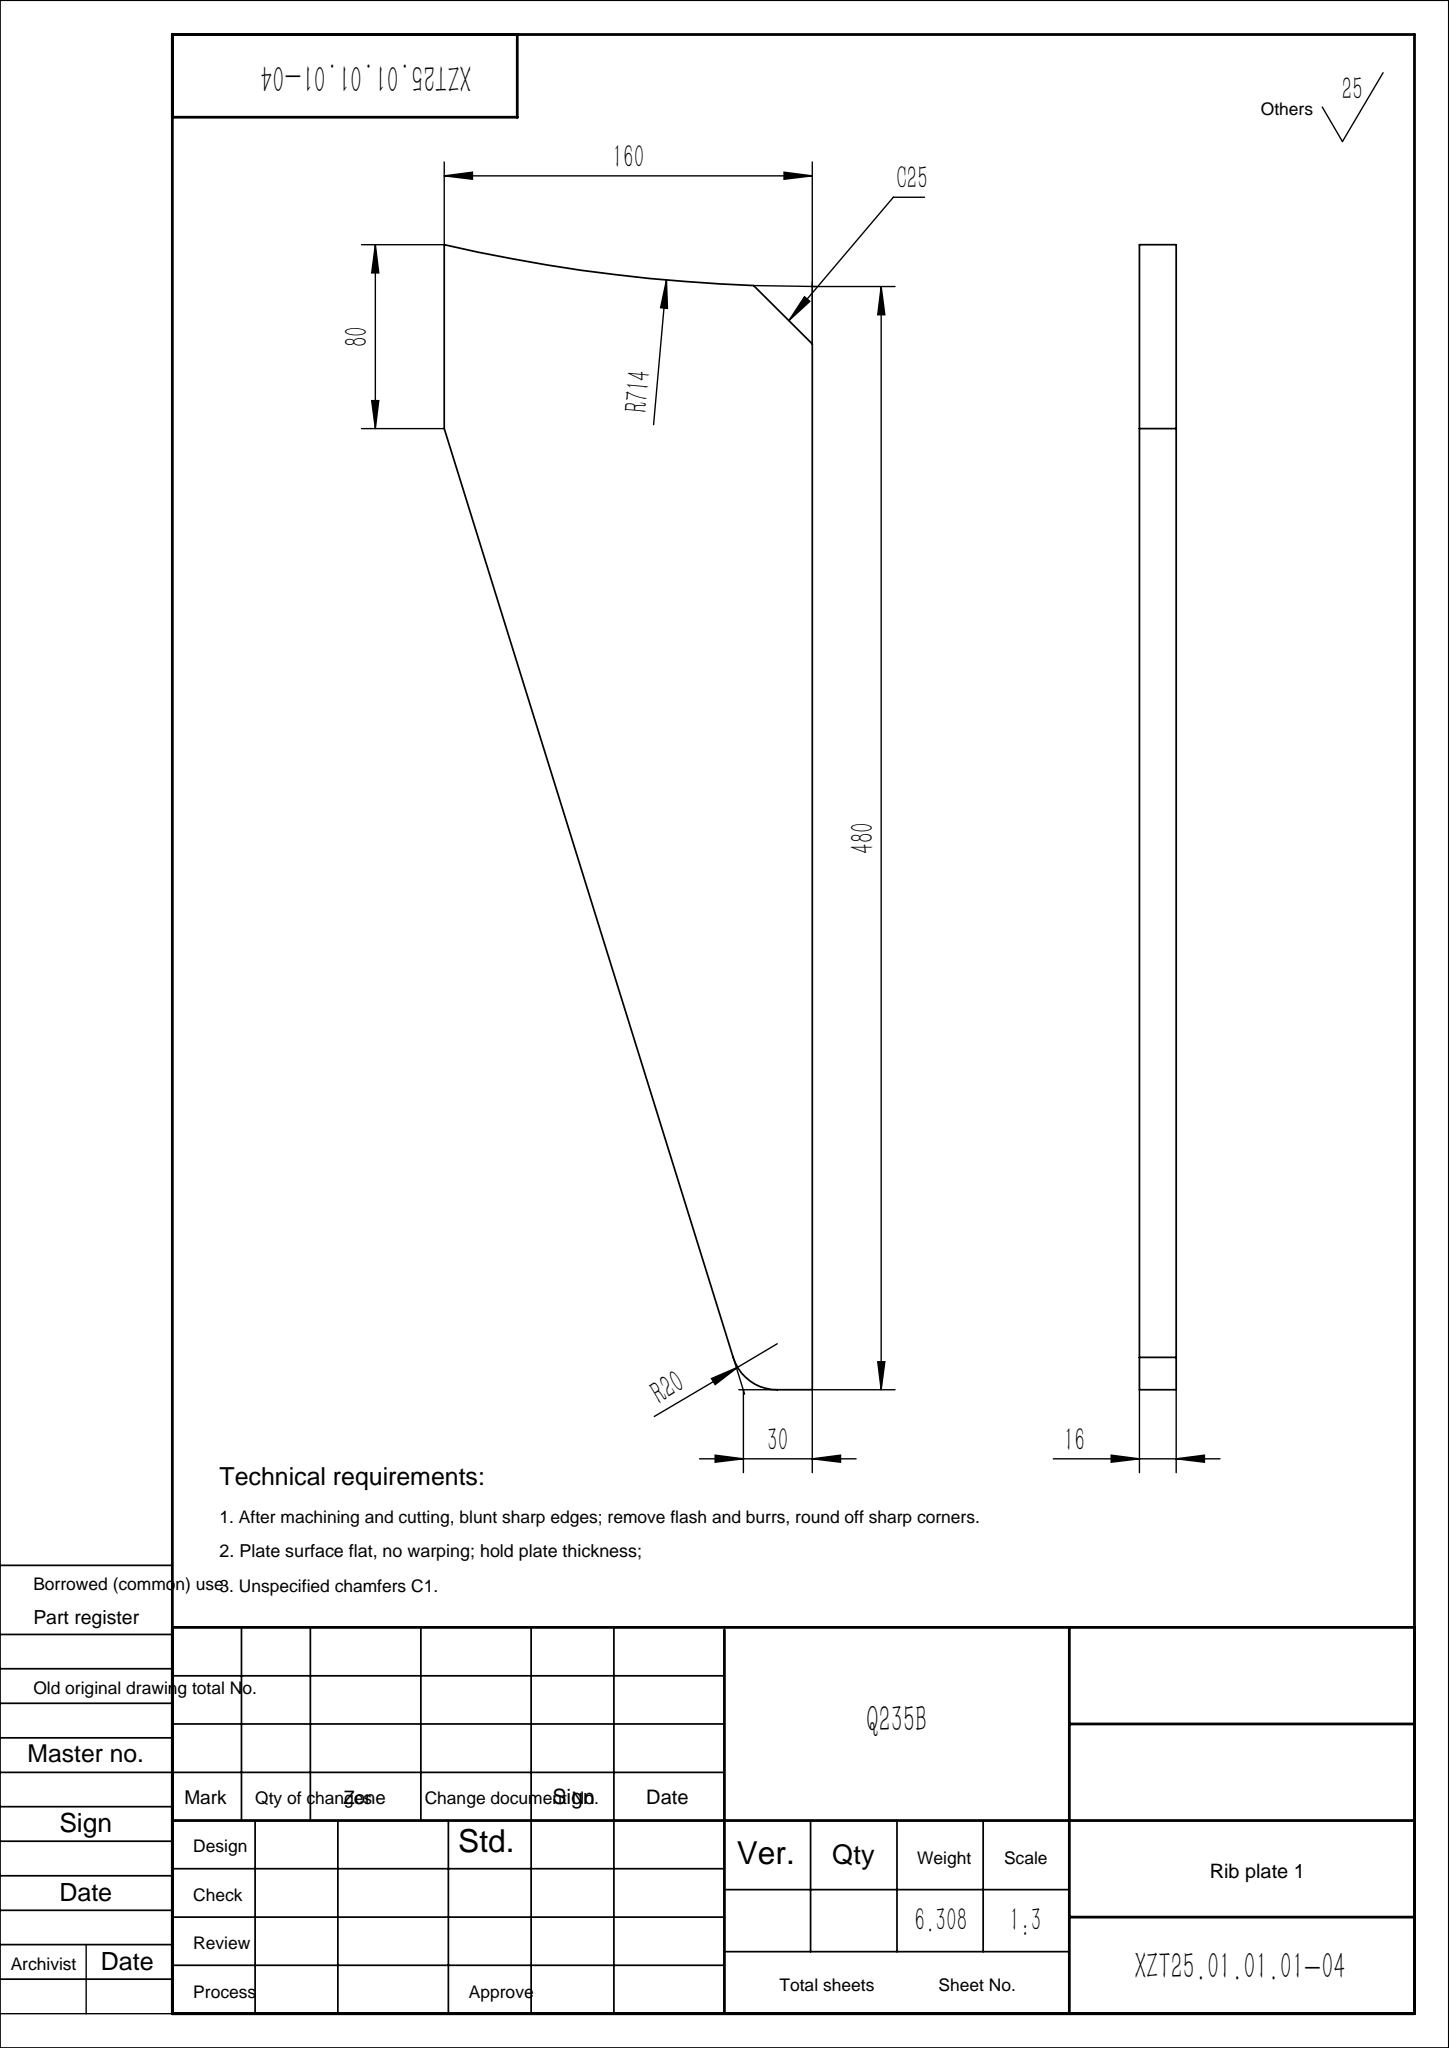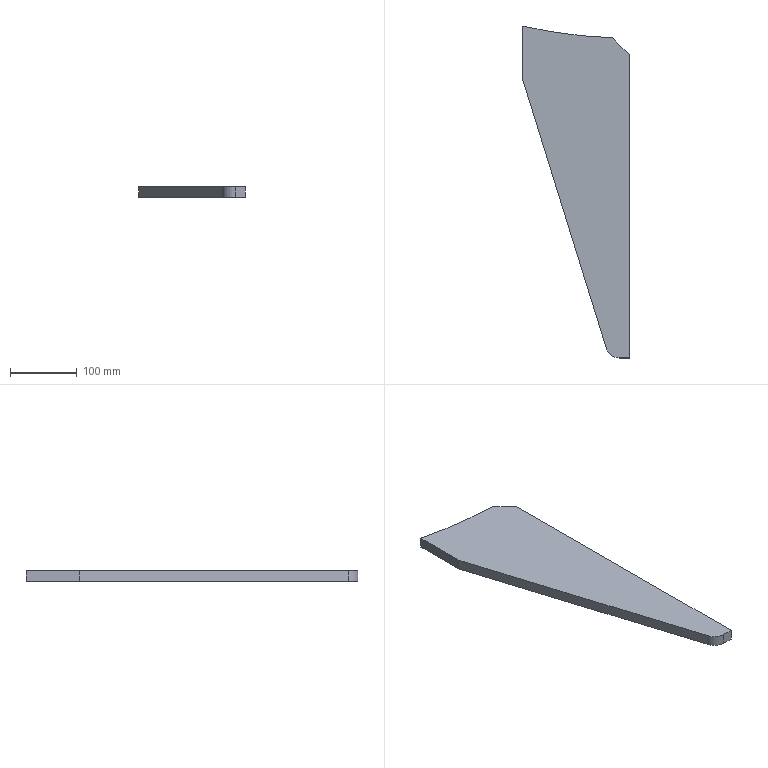Part | SolidWorks | features Chamfer 1, Extrusion 1, Fillet 1 | 1 solid | 9 faces | box 160 x 498.158 x 16 mm | volume 803620 mm3 | plane 7 | cylinder 2 | commonest cylinder face diameters 40 x1 1428 x1
STEP:
#1=CARTESIAN_POINT('',(0.,0.,-8.));
#2=VERTEX_POINT('',#1);
#3=CARTESIAN_POINT('',(0.,455.,-8.));
#4=VERTEX_POINT('',#3);
#5=CARTESIAN_POINT('',(0.,0.,-8.));
#6=DIRECTION('',(0.,1.,0.));
#7=VECTOR('',#6,1000.);
#8=LINE('',#5,#7);
#9=EDGE_CURVE('',#2,#4,#8,.T.);
#10=ORIENTED_EDGE('',*,*,#9,.T.);
#11=CARTESIAN_POINT('',(0.,455.,8.));
#12=VERTEX_POINT('',#11);
#13=CARTESIAN_POINT('',(0.,455.,8.));
#14=DIRECTION('',(0.,0.,1.));
#15=VECTOR('',#14,1000.);
#16=LINE('',#13,#15);
#17=EDGE_CURVE('',#4,#12,#16,.T.);
#18=ORIENTED_EDGE('',*,*,#17,.T.);
#19=CARTESIAN_POINT('',(0.,0.,8.));
#20=VERTEX_POINT('',#19);
#21=CARTESIAN_POINT('',(0.,0.,8.));
#22=DIRECTION('',(0.,1.,0.));
#23=VECTOR('',#22,1000.);
#24=LINE('',#21,#23);
#25=EDGE_CURVE('',#20,#12,#24,.T.);
#26=ORIENTED_EDGE('',*,*,#25,.F.);
#27=CARTESIAN_POINT('',(0.,0.,8.));
#28=DIRECTION('',(0.,0.,-1.));
#29=VECTOR('',#28,1000.);
#30=LINE('',#27,#29);
#31=EDGE_CURVE('',#20,#2,#30,.T.);
#32=ORIENTED_EDGE('',*,*,#31,.T.);
#33=EDGE_LOOP('',(#10,#18,#26,#32));
#34=FACE_OUTER_BOUND('',#33,.T.);
#35=CARTESIAN_POINT('',(0.,0.,8.));
#36=DIRECTION('',(-1.,0.,0.));
#37=DIRECTION('',(0.,0.,1.));
#38=AXIS2_PLACEMENT_3D('',#35,#36,#37);
#39=PLANE('',#38);
#40=ADVANCED_FACE('',(#34),#39,.F.);
#41=CARTESIAN_POINT('',(-25.454,480.454,8.));
#42=VERTEX_POINT('',#41);
#43=CARTESIAN_POINT('',(-160.,498.158,8.));
#44=VERTEX_POINT('',#43);
#45=CARTESIAN_POINT('',(0.,1194.,8.));
#46=DIRECTION('',(0.,0.,-1.));
#47=DIRECTION('',(-1.,0.,0.));
#48=AXIS2_PLACEMENT_3D('',#45,#46,#47);
#49=CIRCLE('',#48,714.);
#50=EDGE_CURVE('',#42,#44,#49,.T.);
#51=ORIENTED_EDGE('',*,*,#50,.F.);
#52=CARTESIAN_POINT('',(-25.454,480.454,-8.));
#53=VERTEX_POINT('',#52);
#54=CARTESIAN_POINT('',(-25.454,480.454,8.));
#55=DIRECTION('',(0.,0.,-1.));
#56=VECTOR('',#55,1000.);
#57=LINE('',#54,#56);
#58=EDGE_CURVE('',#42,#53,#57,.T.);
#59=ORIENTED_EDGE('',*,*,#58,.T.);
#60=CARTESIAN_POINT('',(-160.,498.158,-8.));
#61=VERTEX_POINT('',#60);
#62=CARTESIAN_POINT('',(0.,1194.,-8.));
#63=DIRECTION('',(0.,0.,-1.));
#64=DIRECTION('',(-1.,0.,0.));
#65=AXIS2_PLACEMENT_3D('',#62,#63,#64);
#66=CIRCLE('',#65,714.);
#67=EDGE_CURVE('',#53,#61,#66,.T.);
#68=ORIENTED_EDGE('',*,*,#67,.T.);
#69=CARTESIAN_POINT('',(-160.,498.158,8.));
#70=DIRECTION('',(0.,0.,-1.));
#71=VECTOR('',#70,1000.);
#72=LINE('',#69,#71);
#73=EDGE_CURVE('',#44,#61,#72,.T.);
#74=ORIENTED_EDGE('',*,*,#73,.F.);
#75=EDGE_LOOP('',(#51,#59,#68,#74));
#76=FACE_OUTER_BOUND('',#75,.T.);
#77=CARTESIAN_POINT('',(0.,1194.,8.));
#78=DIRECTION('',(0.,0.,-1.));
#79=DIRECTION('',(-1.,0.,0.));
#80=AXIS2_PLACEMENT_3D('',#77,#78,#79);
#81=CYLINDRICAL_SURFACE('',#80,714.);
#82=ADVANCED_FACE('',(#76),#81,.F.);
#83=CARTESIAN_POINT('',(-160.,418.158,-8.));
#84=VERTEX_POINT('',#83);
#85=CARTESIAN_POINT('',(-160.,418.158,-8.));
#86=DIRECTION('',(0.,-1.,0.));
#87=VECTOR('',#86,1000.);
#88=LINE('',#85,#87);
#89=EDGE_CURVE('',#61,#84,#88,.T.);
#90=ORIENTED_EDGE('',*,*,#89,.T.);
#91=CARTESIAN_POINT('',(-160.,418.158,8.));
#92=VERTEX_POINT('',#91);
#93=CARTESIAN_POINT('',(-160.,418.158,8.));
#94=DIRECTION('',(0.,0.,-1.));
#95=VECTOR('',#94,1000.);
#96=LINE('',#93,#95);
#97=EDGE_CURVE('',#92,#84,#96,.T.);
#98=ORIENTED_EDGE('',*,*,#97,.F.);
#99=CARTESIAN_POINT('',(-160.,418.158,8.));
#100=DIRECTION('',(0.,-1.,0.));
#101=VECTOR('',#100,1000.);
#102=LINE('',#99,#101);
#103=EDGE_CURVE('',#44,#92,#102,.T.);
#104=ORIENTED_EDGE('',*,*,#103,.F.);
#105=ORIENTED_EDGE('',*,*,#73,.T.);
#106=EDGE_LOOP('',(#90,#98,#104,#105));
#107=FACE_OUTER_BOUND('',#106,.T.);
#108=CARTESIAN_POINT('',(-160.,418.158,8.));
#109=DIRECTION('',(1.,0.,0.));
#110=DIRECTION('',(0.,1.,0.));
#111=AXIS2_PLACEMENT_3D('',#108,#109,#110);
#112=PLANE('',#111);
#113=ADVANCED_FACE('',(#107),#112,.F.);
#114=CARTESIAN_POINT('',(-34.372,14.063,-8.));
#115=VERTEX_POINT('',#114);
#116=CARTESIAN_POINT('',(-30.,0.,-8.));
#117=DIRECTION('',(0.2969,-0.9549,0.));
#118=VECTOR('',#117,1000.);
#119=LINE('',#116,#118);
#120=EDGE_CURVE('',#84,#115,#119,.T.);
#121=ORIENTED_EDGE('',*,*,#120,.T.);
#122=CARTESIAN_POINT('',(-34.372,14.063,8.));
#123=VERTEX_POINT('',#122);
#124=CARTESIAN_POINT('',(-34.372,14.063,8.));
#125=DIRECTION('',(0.,0.,1.));
#126=VECTOR('',#125,1000.);
#127=LINE('',#124,#126);
#128=EDGE_CURVE('',#115,#123,#127,.T.);
#129=ORIENTED_EDGE('',*,*,#128,.T.);
#130=CARTESIAN_POINT('',(-30.,0.,8.));
#131=DIRECTION('',(0.2969,-0.9549,0.));
#132=VECTOR('',#131,1000.);
#133=LINE('',#130,#132);
#134=EDGE_CURVE('',#92,#123,#133,.T.);
#135=ORIENTED_EDGE('',*,*,#134,.F.);
#136=ORIENTED_EDGE('',*,*,#97,.T.);
#137=EDGE_LOOP('',(#121,#129,#135,#136));
#138=FACE_OUTER_BOUND('',#137,.T.);
#139=CARTESIAN_POINT('',(-30.,0.,8.));
#140=DIRECTION('',(0.9549,0.2969,0.));
#141=DIRECTION('',(-0.2969,0.9549,0.));
#142=AXIS2_PLACEMENT_3D('',#139,#140,#141);
#143=PLANE('',#142);
#144=ADVANCED_FACE('',(#138),#143,.F.);
#145=CARTESIAN_POINT('',(-15.274,0.,8.));
#146=VERTEX_POINT('',#145);
#147=CARTESIAN_POINT('',(0.,0.,8.));
#148=DIRECTION('',(1.,0.,0.));
#149=VECTOR('',#148,1000.);
#150=LINE('',#147,#149);
#151=EDGE_CURVE('',#146,#20,#150,.T.);
#152=ORIENTED_EDGE('',*,*,#151,.F.);
#153=CARTESIAN_POINT('',(-15.274,0.,-8.));
#154=VERTEX_POINT('',#153);
#155=CARTESIAN_POINT('',(-15.274,0.,8.));
#156=DIRECTION('',(0.,0.,-1.));
#157=VECTOR('',#156,1000.);
#158=LINE('',#155,#157);
#159=EDGE_CURVE('',#146,#154,#158,.T.);
#160=ORIENTED_EDGE('',*,*,#159,.T.);
#161=CARTESIAN_POINT('',(0.,0.,-8.));
#162=DIRECTION('',(1.,0.,0.));
#163=VECTOR('',#162,1000.);
#164=LINE('',#161,#163);
#165=EDGE_CURVE('',#154,#2,#164,.T.);
#166=ORIENTED_EDGE('',*,*,#165,.T.);
#167=ORIENTED_EDGE('',*,*,#31,.F.);
#168=EDGE_LOOP('',(#152,#160,#166,#167));
#169=FACE_OUTER_BOUND('',#168,.T.);
#170=CARTESIAN_POINT('',(0.,0.,8.));
#171=DIRECTION('',(0.,1.,0.));
#172=DIRECTION('',(-1.,0.,0.));
#173=AXIS2_PLACEMENT_3D('',#170,#171,#172);
#174=PLANE('',#173);
#175=ADVANCED_FACE('',(#169),#174,.F.);
#176=ORIENTED_EDGE('',*,*,#25,.T.);
#177=CARTESIAN_POINT('',(-25.454,480.454,8.));
#178=DIRECTION('',(-0.7071,0.7071,0.));
#179=VECTOR('',#178,1000.);
#180=LINE('',#177,#179);
#181=EDGE_CURVE('',#12,#42,#180,.T.);
#182=ORIENTED_EDGE('',*,*,#181,.T.);
#183=ORIENTED_EDGE('',*,*,#50,.T.);
#184=ORIENTED_EDGE('',*,*,#103,.T.);
#185=ORIENTED_EDGE('',*,*,#134,.T.);
#186=CARTESIAN_POINT('',(-15.274,20.,8.));
#187=DIRECTION('',(0.,0.,1.));
#188=DIRECTION('',(-1.,0.,0.));
#189=AXIS2_PLACEMENT_3D('',#186,#187,#188);
#190=CIRCLE('',#189,20.);
#191=EDGE_CURVE('',#123,#146,#190,.T.);
#192=ORIENTED_EDGE('',*,*,#191,.T.);
#193=ORIENTED_EDGE('',*,*,#151,.T.);
#194=EDGE_LOOP('',(#176,#182,#183,#184,#185,#192,#193));
#195=FACE_OUTER_BOUND('',#194,.T.);
#196=CARTESIAN_POINT('',(0.,1194.,8.));
#197=DIRECTION('',(0.,0.,-1.));
#198=DIRECTION('',(-1.,0.,0.));
#199=AXIS2_PLACEMENT_3D('',#196,#197,#198);
#200=PLANE('',#199);
#201=ADVANCED_FACE('',(#195),#200,.F.);
#202=ORIENTED_EDGE('',*,*,#67,.F.);
#203=CARTESIAN_POINT('',(-369.5,824.5,-8.));
#204=DIRECTION('',(0.7071,-0.7071,0.));
#205=VECTOR('',#204,1000.);
#206=LINE('',#203,#205);
#207=EDGE_CURVE('',#53,#4,#206,.T.);
#208=ORIENTED_EDGE('',*,*,#207,.T.);
#209=ORIENTED_EDGE('',*,*,#9,.F.);
#210=ORIENTED_EDGE('',*,*,#165,.F.);
#211=CARTESIAN_POINT('',(-15.274,20.,-8.));
#212=DIRECTION('',(0.,0.,-1.));
#213=DIRECTION('',(-1.,0.,0.));
#214=AXIS2_PLACEMENT_3D('',#211,#212,#213);
#215=CIRCLE('',#214,20.);
#216=EDGE_CURVE('',#154,#115,#215,.T.);
#217=ORIENTED_EDGE('',*,*,#216,.T.);
#218=ORIENTED_EDGE('',*,*,#120,.F.);
#219=ORIENTED_EDGE('',*,*,#89,.F.);
#220=EDGE_LOOP('',(#202,#208,#209,#210,#217,#218,#219));
#221=FACE_OUTER_BOUND('',#220,.T.);
#222=CARTESIAN_POINT('',(0.,1194.,-8.));
#223=DIRECTION('',(0.,0.,-1.));
#224=DIRECTION('',(-1.,0.,0.));
#225=AXIS2_PLACEMENT_3D('',#222,#223,#224);
#226=PLANE('',#225);
#227=ADVANCED_FACE('',(#221),#226,.T.);
#228=ORIENTED_EDGE('',*,*,#191,.F.);
#229=ORIENTED_EDGE('',*,*,#128,.F.);
#230=ORIENTED_EDGE('',*,*,#216,.F.);
#231=ORIENTED_EDGE('',*,*,#159,.F.);
#232=EDGE_LOOP('',(#228,#229,#230,#231));
#233=FACE_OUTER_BOUND('',#232,.T.);
#234=CARTESIAN_POINT('',(-15.274,20.,8.));
#235=DIRECTION('',(0.,0.,-1.));
#236=DIRECTION('',(-1.,0.,0.));
#237=AXIS2_PLACEMENT_3D('',#234,#235,#236);
#238=CYLINDRICAL_SURFACE('',#237,20.);
#239=ADVANCED_FACE('',(#233),#238,.T.);
#240=ORIENTED_EDGE('',*,*,#181,.F.);
#241=ORIENTED_EDGE('',*,*,#17,.F.);
#242=ORIENTED_EDGE('',*,*,#207,.F.);
#243=ORIENTED_EDGE('',*,*,#58,.F.);
#244=EDGE_LOOP('',(#240,#241,#242,#243));
#245=FACE_OUTER_BOUND('',#244,.T.);
#246=CARTESIAN_POINT('',(-25.454,480.454,8.));
#247=DIRECTION('',(-0.7071,-0.7071,0.));
#248=DIRECTION('',(0.,0.,-1.));
#249=AXIS2_PLACEMENT_3D('',#246,#247,#248);
#250=PLANE('',#249);
#251=ADVANCED_FACE('',(#245),#250,.F.);
#252=CLOSED_SHELL('',(#40,#82,#113,#144,#175,#201,#227,#239,#251));
#253=MANIFOLD_SOLID_BREP('',#252);
#254=CARTESIAN_POINT('',(0.,0.,0.));
#255=DIRECTION('',(0.,0.,1.));
#256=DIRECTION('',(1.,0.,0.));
#257=AXIS2_PLACEMENT_3D('',#254,#255,#256);
#258=(LENGTH_UNIT()NAMED_UNIT(*)SI_UNIT(.MILLI.,.METRE.));
#259=UNCERTAINTY_MEASURE_WITH_UNIT(LENGTH_MEASURE(0.00001),#258,'','');
#260=(NAMED_UNIT(*)PLANE_ANGLE_UNIT()SI_UNIT($,.RADIAN.));
#261=(NAMED_UNIT(*)SI_UNIT($,.STERADIAN.)SOLID_ANGLE_UNIT());
#262=(GEOMETRIC_REPRESENTATION_CONTEXT(3)GLOBAL_UNCERTAINTY_ASSIGNED_CONTEXT((#259))GLOBAL_UNIT_ASSIGNED_CONTEXT((#258,#260,#261))REPRESENTATION_CONTEXT('',''));
#263=ADVANCED_BREP_SHAPE_REPRESENTATION('',(#253,#257),#262);